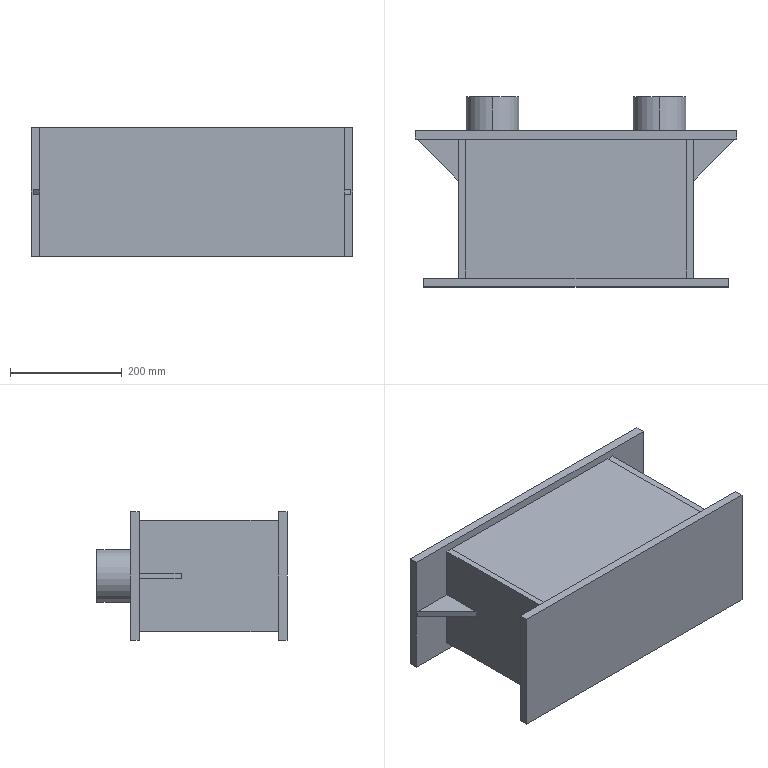Part | STEP file | Spring lower seat 2_Default<As machined> | 10 solids | 58 faces | box 575.505 x 341 x 230 mm | volume 7946213 mm3 | plane 50 | cylinder 8 | commonest cylinder face diameters 83 x4 95 x4